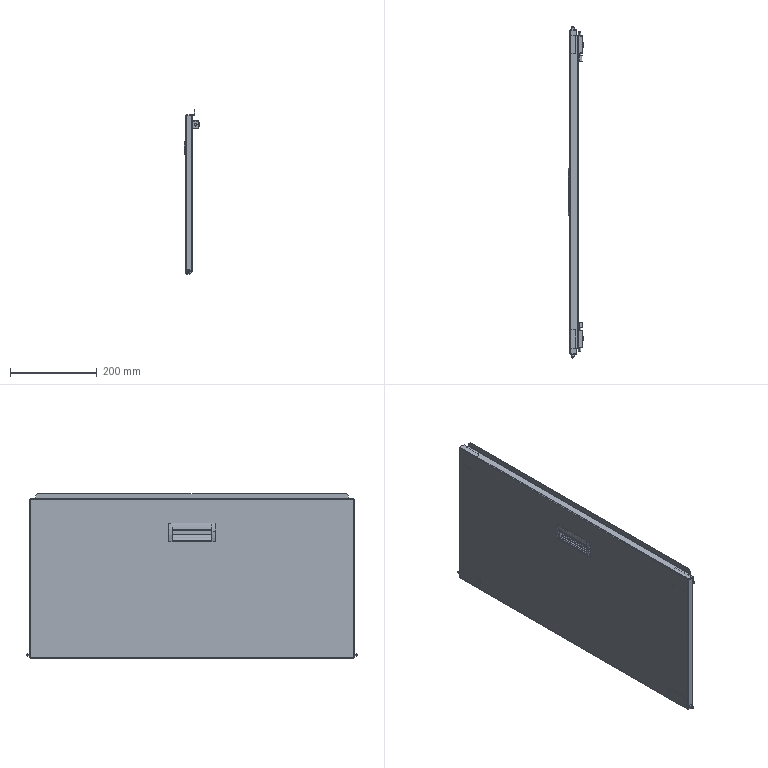Part | SolidWorks | 16 solids | 429 faces | box 35.649 x 764 x 379.5 mm | volume 533274 mm3 | plane 243 | cylinder 174 | cone 8 | torus 4 | commonest cylinder face diameters 1 x18 2.5 x16 3.2 x16 0.6 x14 7 x13 2 x8